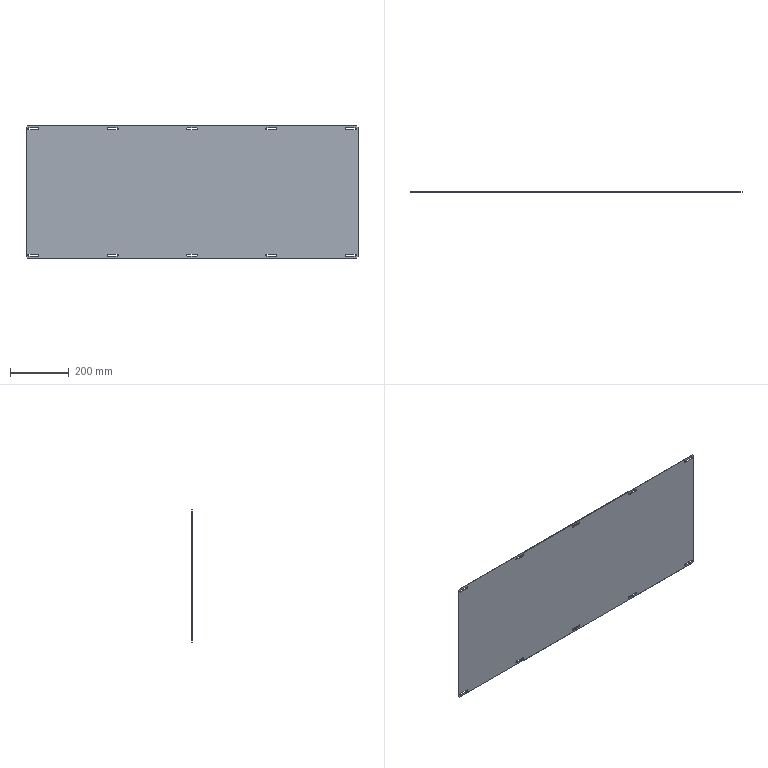Part | NX | features BREP 1 | 1 solid | 50 faces | box 1130 x 1.5 x 450 mm | volume 758948 mm3 | plane 30 | cylinder 20 | commonest cylinder face diameters 7 x20